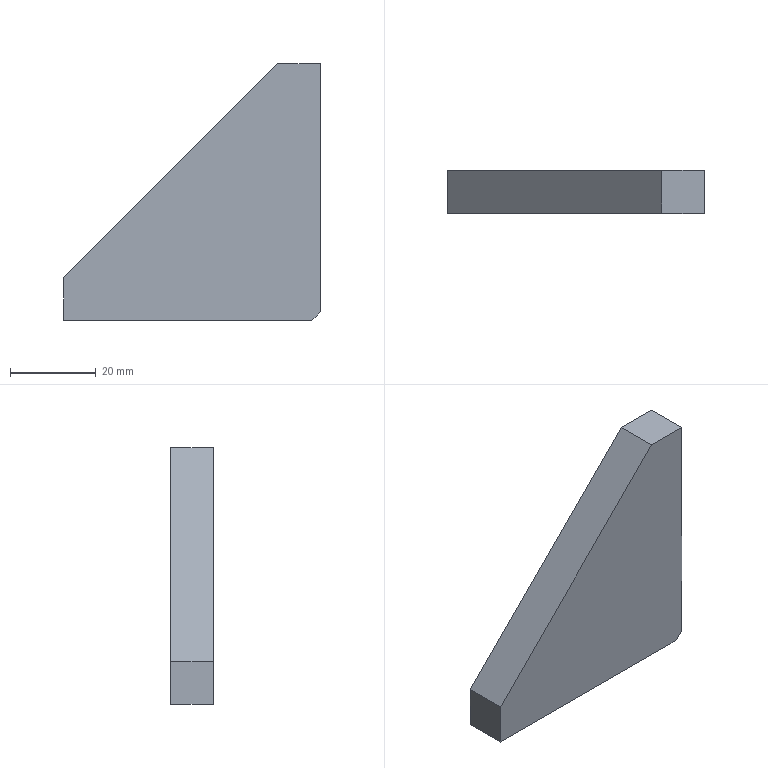Part | STEP file | PN_0011 | 1 solid | 24 faces | box 60 x 10 x 60 mm | volume 22770 mm3 | cylinder 8 | cone 8 | plane 8 | commonest cylinder face diameters 4.2 x8